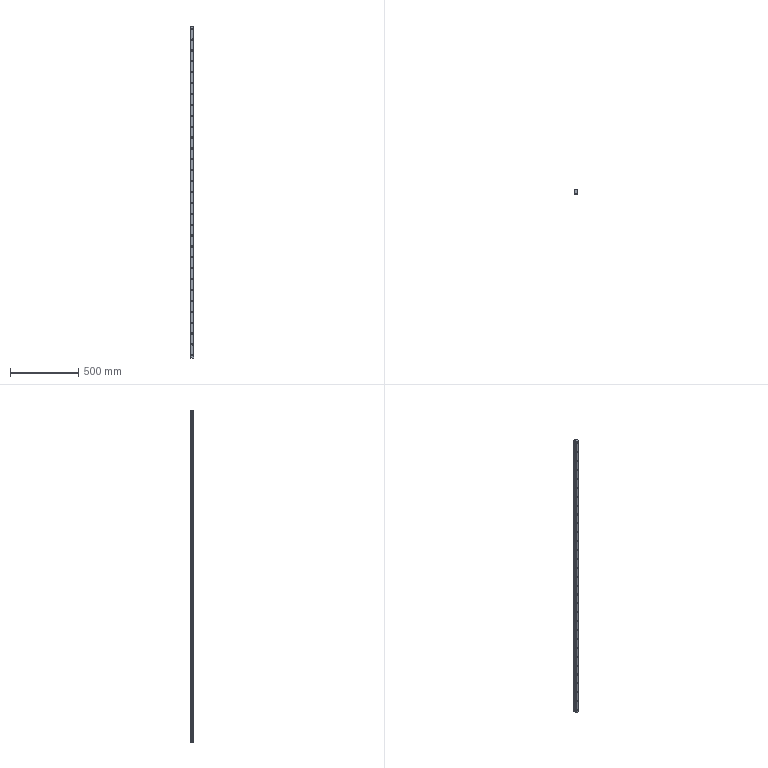Part | SolidWorks | features BaseBody 1 | 1 solid | 254 faces | box 28 x 26 x 2440 mm | volume 1485558 mm3 | cylinder 161 | plane 93 | commonest cylinder face diameters 9 x62 14 x62 1.152 x10 1.613 x8 0.922 x7 1.383 x4